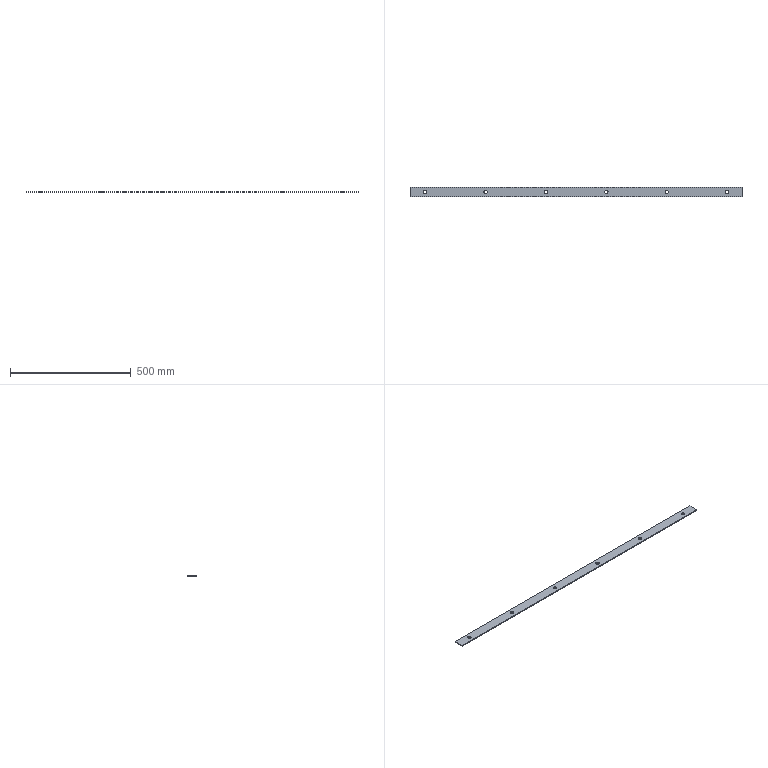Part | STEP file | Pressure plate 2_Default<As machined> | 1 solid | 18 faces | box 1374 x 40 x 4 mm | volume 216145 mm3 | cylinder 12 | plane 6 | commonest cylinder face diameters 14 x12
STEP:
#1=CARTESIAN_POINT('',(0.,0.,0.));
#2=DIRECTION('',(0.,0.,1.));
#3=DIRECTION('',(1.,0.,0.));
#4=AXIS2_PLACEMENT_3D('',#1,#2,#3);
#5=CARTESIAN_POINT('',(618.5,-541.136,4.));
#6=VERTEX_POINT('',#5);
#7=CARTESIAN_POINT('',(618.5,-541.136,0.));
#8=VERTEX_POINT('',#7);
#9=CARTESIAN_POINT('',(618.5,-541.136,4.));
#10=DIRECTION('',(0.,0.,-1.));
#11=VECTOR('',#10,1.);
#12=LINE('',#9,#11);
#13=CARTESIAN_POINT('',(625.5,-541.136,4.));
#14=DIRECTION('',(0.,0.,-1.));
#15=DIRECTION('',(-1.,0.,0.));
#16=AXIS2_PLACEMENT_3D('',#13,#14,#15);
#17=CYLINDRICAL_SURFACE('',#16,7.);
#18=CARTESIAN_POINT('',(6.283,0.));
#19=DIRECTION('',(0.,1.));
#20=VECTOR('',#19,1.);
#21=LINE('',#18,#20);
#22=(GEOMETRIC_REPRESENTATION_CONTEXT(2)PARAMETRIC_REPRESENTATION_CONTEXT()REPRESENTATION_CONTEXT('',''));
#23=DEFINITIONAL_REPRESENTATION('',(#21),#22);
#24=PCURVE('',#17,#23);
#25=CARTESIAN_POINT('',(625.5,-541.136,4.));
#26=DIRECTION('',(0.,0.,-1.));
#27=DIRECTION('',(-1.,0.,0.));
#28=AXIS2_PLACEMENT_3D('',#25,#26,#27);
#29=CYLINDRICAL_SURFACE('',#28,7.);
#30=CARTESIAN_POINT('',(0.,0.));
#31=DIRECTION('',(0.,1.));
#32=VECTOR('',#31,1.);
#33=LINE('',#30,#32);
#34=(GEOMETRIC_REPRESENTATION_CONTEXT(2)PARAMETRIC_REPRESENTATION_CONTEXT()REPRESENTATION_CONTEXT('',''));
#35=DEFINITIONAL_REPRESENTATION('',(#33),#34);
#36=PCURVE('',#29,#35);
#37=SURFACE_CURVE('',#12,(#24,#36),.PCURVE_S1.);
#38=EDGE_CURVE('',#6,#8,#37,.T.);
#39=ORIENTED_EDGE('',*,*,#38,.T.);
#40=CARTESIAN_POINT('',(632.5,-541.136,0.));
#41=VERTEX_POINT('',#40);
#42=CARTESIAN_POINT('',(625.5,-541.136,0.));
#43=DIRECTION('',(0.,0.,1.));
#44=DIRECTION('',(1.,0.,0.));
#45=AXIS2_PLACEMENT_3D('',#42,#43,#44);
#46=CIRCLE('',#45,7.);
#47=CARTESIAN_POINT('',(9.425,4.));
#48=DIRECTION('',(-1.,0.));
#49=VECTOR('',#48,1.);
#50=LINE('',#47,#49);
#51=(GEOMETRIC_REPRESENTATION_CONTEXT(2)PARAMETRIC_REPRESENTATION_CONTEXT()REPRESENTATION_CONTEXT('',''));
#52=DEFINITIONAL_REPRESENTATION('',(#50),#51);
#53=PCURVE('',#17,#52);
#54=CARTESIAN_POINT('',(0.,0.,0.));
#55=DIRECTION('',(0.,0.,1.));
#56=DIRECTION('',(1.,0.,0.));
#57=AXIS2_PLACEMENT_3D('',#54,#55,#56);
#58=PLANE('',#57);
#59=CARTESIAN_POINT('',(625.5,-541.136));
#60=DIRECTION('',(1.,0.));
#61=AXIS2_PLACEMENT_2D('',#59,#60);
#62=CIRCLE('',#61,7.);
#63=(GEOMETRIC_REPRESENTATION_CONTEXT(2)PARAMETRIC_REPRESENTATION_CONTEXT()REPRESENTATION_CONTEXT('',''));
#64=DEFINITIONAL_REPRESENTATION('',(#62),#63);
#65=PCURVE('',#58,#64);
#66=SURFACE_CURVE('',#46,(#53,#65),.PCURVE_S1.);
#67=EDGE_CURVE('',#8,#41,#66,.T.);
#68=ORIENTED_EDGE('',*,*,#67,.T.);
#69=CARTESIAN_POINT('',(632.5,-541.136,4.));
#70=VERTEX_POINT('',#69);
#71=CARTESIAN_POINT('',(632.5,-541.136,4.));
#72=DIRECTION('',(0.,0.,-1.));
#73=VECTOR('',#72,1.);
#74=LINE('',#71,#73);
#75=CARTESIAN_POINT('',(3.142,0.));
#76=DIRECTION('',(0.,1.));
#77=VECTOR('',#76,1.);
#78=LINE('',#75,#77);
#79=(GEOMETRIC_REPRESENTATION_CONTEXT(2)PARAMETRIC_REPRESENTATION_CONTEXT()REPRESENTATION_CONTEXT('',''));
#80=DEFINITIONAL_REPRESENTATION('',(#78),#79);
#81=PCURVE('',#17,#80);
#82=CARTESIAN_POINT('',(3.142,0.));
#83=DIRECTION('',(0.,1.));
#84=VECTOR('',#83,1.);
#85=LINE('',#82,#84);
#86=(GEOMETRIC_REPRESENTATION_CONTEXT(2)PARAMETRIC_REPRESENTATION_CONTEXT()REPRESENTATION_CONTEXT('',''));
#87=DEFINITIONAL_REPRESENTATION('',(#85),#86);
#88=PCURVE('',#29,#87);
#89=SURFACE_CURVE('',#74,(#81,#88),.PCURVE_S1.);
#90=EDGE_CURVE('',#70,#41,#89,.T.);
#91=ORIENTED_EDGE('',*,*,#90,.F.);
#92=CARTESIAN_POINT('',(625.5,-541.136,4.));
#93=DIRECTION('',(0.,0.,1.));
#94=DIRECTION('',(1.,0.,0.));
#95=AXIS2_PLACEMENT_3D('',#92,#93,#94);
#96=CIRCLE('',#95,7.);
#97=CARTESIAN_POINT('',(9.425,0.));
#98=DIRECTION('',(-1.,0.));
#99=VECTOR('',#98,1.);
#100=LINE('',#97,#99);
#101=(GEOMETRIC_REPRESENTATION_CONTEXT(2)PARAMETRIC_REPRESENTATION_CONTEXT()REPRESENTATION_CONTEXT('',''));
#102=DEFINITIONAL_REPRESENTATION('',(#100),#101);
#103=PCURVE('',#17,#102);
#104=CARTESIAN_POINT('',(0.,0.,4.));
#105=DIRECTION('',(0.,0.,1.));
#106=DIRECTION('',(1.,0.,0.));
#107=AXIS2_PLACEMENT_3D('',#104,#105,#106);
#108=PLANE('',#107);
#109=CARTESIAN_POINT('',(625.5,-541.136));
#110=DIRECTION('',(1.,0.));
#111=AXIS2_PLACEMENT_2D('',#109,#110);
#112=CIRCLE('',#111,7.);
#113=(GEOMETRIC_REPRESENTATION_CONTEXT(2)PARAMETRIC_REPRESENTATION_CONTEXT()REPRESENTATION_CONTEXT('',''));
#114=DEFINITIONAL_REPRESENTATION('',(#112),#113);
#115=PCURVE('',#108,#114);
#116=SURFACE_CURVE('',#96,(#103,#115),.PCURVE_S1.);
#117=EDGE_CURVE('',#6,#70,#116,.T.);
#118=ORIENTED_EDGE('',*,*,#117,.F.);
#119=EDGE_LOOP('',(#39,#68,#91,#118));
#120=FACE_BOUND('',#119,.F.);
#121=ADVANCED_FACE('',(#120),#17,.F.);
#122=CARTESIAN_POINT('',(368.5,-541.136,4.));
#123=VERTEX_POINT('',#122);
#124=CARTESIAN_POINT('',(368.5,-541.136,0.));
#125=VERTEX_POINT('',#124);
#126=CARTESIAN_POINT('',(368.5,-541.136,4.));
#127=DIRECTION('',(0.,0.,-1.));
#128=VECTOR('',#127,1.);
#129=LINE('',#126,#128);
#130=CARTESIAN_POINT('',(375.5,-541.136,4.));
#131=DIRECTION('',(0.,0.,-1.));
#132=DIRECTION('',(-1.,0.,0.));
#133=AXIS2_PLACEMENT_3D('',#130,#131,#132);
#134=CYLINDRICAL_SURFACE('',#133,7.);
#135=CARTESIAN_POINT('',(6.283,0.));
#136=DIRECTION('',(0.,1.));
#137=VECTOR('',#136,1.);
#138=LINE('',#135,#137);
#139=(GEOMETRIC_REPRESENTATION_CONTEXT(2)PARAMETRIC_REPRESENTATION_CONTEXT()REPRESENTATION_CONTEXT('',''));
#140=DEFINITIONAL_REPRESENTATION('',(#138),#139);
#141=PCURVE('',#134,#140);
#142=CARTESIAN_POINT('',(375.5,-541.136,4.));
#143=DIRECTION('',(0.,0.,-1.));
#144=DIRECTION('',(-1.,0.,0.));
#145=AXIS2_PLACEMENT_3D('',#142,#143,#144);
#146=CYLINDRICAL_SURFACE('',#145,7.);
#147=CARTESIAN_POINT('',(0.,0.));
#148=DIRECTION('',(0.,1.));
#149=VECTOR('',#148,1.);
#150=LINE('',#147,#149);
#151=(GEOMETRIC_REPRESENTATION_CONTEXT(2)PARAMETRIC_REPRESENTATION_CONTEXT()REPRESENTATION_CONTEXT('',''));
#152=DEFINITIONAL_REPRESENTATION('',(#150),#151);
#153=PCURVE('',#146,#152);
#154=SURFACE_CURVE('',#129,(#141,#153),.PCURVE_S1.);
#155=EDGE_CURVE('',#123,#125,#154,.T.);
#156=ORIENTED_EDGE('',*,*,#155,.T.);
#157=CARTESIAN_POINT('',(382.5,-541.136,0.));
#158=VERTEX_POINT('',#157);
#159=CARTESIAN_POINT('',(375.5,-541.136,0.));
#160=DIRECTION('',(0.,0.,1.));
#161=DIRECTION('',(1.,0.,0.));
#162=AXIS2_PLACEMENT_3D('',#159,#160,#161);
#163=CIRCLE('',#162,7.);
#164=CARTESIAN_POINT('',(9.425,4.));
#165=DIRECTION('',(-1.,0.));
#166=VECTOR('',#165,1.);
#167=LINE('',#164,#166);
#168=(GEOMETRIC_REPRESENTATION_CONTEXT(2)PARAMETRIC_REPRESENTATION_CONTEXT()REPRESENTATION_CONTEXT('',''));
#169=DEFINITIONAL_REPRESENTATION('',(#167),#168);
#170=PCURVE('',#134,#169);
#171=CARTESIAN_POINT('',(375.5,-541.136));
#172=DIRECTION('',(1.,0.));
#173=AXIS2_PLACEMENT_2D('',#171,#172);
#174=CIRCLE('',#173,7.);
#175=(GEOMETRIC_REPRESENTATION_CONTEXT(2)PARAMETRIC_REPRESENTATION_CONTEXT()REPRESENTATION_CONTEXT('',''));
#176=DEFINITIONAL_REPRESENTATION('',(#174),#175);
#177=PCURVE('',#58,#176);
#178=SURFACE_CURVE('',#163,(#170,#177),.PCURVE_S1.);
#179=EDGE_CURVE('',#125,#158,#178,.T.);
#180=ORIENTED_EDGE('',*,*,#179,.T.);
#181=CARTESIAN_POINT('',(382.5,-541.136,4.));
#182=VERTEX_POINT('',#181);
#183=CARTESIAN_POINT('',(382.5,-541.136,4.));
#184=DIRECTION('',(0.,0.,-1.));
#185=VECTOR('',#184,1.);
#186=LINE('',#183,#185);
#187=CARTESIAN_POINT('',(3.142,0.));
#188=DIRECTION('',(0.,1.));
#189=VECTOR('',#188,1.);
#190=LINE('',#187,#189);
#191=(GEOMETRIC_REPRESENTATION_CONTEXT(2)PARAMETRIC_REPRESENTATION_CONTEXT()REPRESENTATION_CONTEXT('',''));
#192=DEFINITIONAL_REPRESENTATION('',(#190),#191);
#193=PCURVE('',#134,#192);
#194=CARTESIAN_POINT('',(3.142,0.));
#195=DIRECTION('',(0.,1.));
#196=VECTOR('',#195,1.);
#197=LINE('',#194,#196);
#198=(GEOMETRIC_REPRESENTATION_CONTEXT(2)PARAMETRIC_REPRESENTATION_CONTEXT()REPRESENTATION_CONTEXT('',''));
#199=DEFINITIONAL_REPRESENTATION('',(#197),#198);
#200=PCURVE('',#146,#199);
#201=SURFACE_CURVE('',#186,(#193,#200),.PCURVE_S1.);
#202=EDGE_CURVE('',#182,#158,#201,.T.);
#203=ORIENTED_EDGE('',*,*,#202,.F.);
#204=CARTESIAN_POINT('',(375.5,-541.136,4.));
#205=DIRECTION('',(0.,0.,1.));
#206=DIRECTION('',(1.,0.,0.));
#207=AXIS2_PLACEMENT_3D('',#204,#205,#206);
#208=CIRCLE('',#207,7.);
#209=CARTESIAN_POINT('',(9.425,0.));
#210=DIRECTION('',(-1.,0.));
#211=VECTOR('',#210,1.);
#212=LINE('',#209,#211);
#213=(GEOMETRIC_REPRESENTATION_CONTEXT(2)PARAMETRIC_REPRESENTATION_CONTEXT()REPRESENTATION_CONTEXT('',''));
#214=DEFINITIONAL_REPRESENTATION('',(#212),#213);
#215=PCURVE('',#134,#214);
#216=CARTESIAN_POINT('',(375.5,-541.136));
#217=DIRECTION('',(1.,0.));
#218=AXIS2_PLACEMENT_2D('',#216,#217);
#219=CIRCLE('',#218,7.);
#220=(GEOMETRIC_REPRESENTATION_CONTEXT(2)PARAMETRIC_REPRESENTATION_CONTEXT()REPRESENTATION_CONTEXT('',''));
#221=DEFINITIONAL_REPRESENTATION('',(#219),#220);
#222=PCURVE('',#108,#221);
#223=SURFACE_CURVE('',#208,(#215,#222),.PCURVE_S1.);
#224=EDGE_CURVE('',#123,#182,#223,.T.);
#225=ORIENTED_EDGE('',*,*,#224,.F.);
#226=EDGE_LOOP('',(#156,#180,#203,#225));
#227=FACE_BOUND('',#226,.F.);
#228=ADVANCED_FACE('',(#227),#134,.F.);
#229=CARTESIAN_POINT('',(118.5,-541.136,4.));
#230=VERTEX_POINT('',#229);
#231=CARTESIAN_POINT('',(118.5,-541.136,0.));
#232=VERTEX_POINT('',#231);
#233=CARTESIAN_POINT('',(118.5,-541.136,4.));
#234=DIRECTION('',(0.,0.,-1.));
#235=VECTOR('',#234,1.);
#236=LINE('',#233,#235);
#237=CARTESIAN_POINT('',(125.5,-541.136,4.));
#238=DIRECTION('',(0.,0.,-1.));
#239=DIRECTION('',(-1.,0.,0.));
#240=AXIS2_PLACEMENT_3D('',#237,#238,#239);
#241=CYLINDRICAL_SURFACE('',#240,7.);
#242=CARTESIAN_POINT('',(6.283,0.));
#243=DIRECTION('',(0.,1.));
#244=VECTOR('',#243,1.);
#245=LINE('',#242,#244);
#246=(GEOMETRIC_REPRESENTATION_CONTEXT(2)PARAMETRIC_REPRESENTATION_CONTEXT()REPRESENTATION_CONTEXT('',''));
#247=DEFINITIONAL_REPRESENTATION('',(#245),#246);
#248=PCURVE('',#241,#247);
#249=CARTESIAN_POINT('',(125.5,-541.136,4.));
#250=DIRECTION('',(0.,0.,-1.));
#251=DIRECTION('',(-1.,0.,0.));
#252=AXIS2_PLACEMENT_3D('',#249,#250,#251);
#253=CYLINDRICAL_SURFACE('',#252,7.);
#254=CARTESIAN_POINT('',(0.,0.));
#255=DIRECTION('',(0.,1.));
#256=VECTOR('',#255,1.);
#257=LINE('',#254,#256);
#258=(GEOMETRIC_REPRESENTATION_CONTEXT(2)PARAMETRIC_REPRESENTATION_CONTEXT()REPRESENTATION_CONTEXT('',''));
#259=DEFINITIONAL_REPRESENTATION('',(#257),#258);
#260=PCURVE('',#253,#259);
#261=SURFACE_CURVE('',#236,(#248,#260),.PCURVE_S1.);
#262=EDGE_CURVE('',#230,#232,#261,.T.);
#263=ORIENTED_EDGE('',*,*,#262,.T.);
#264=CARTESIAN_POINT('',(132.5,-541.136,0.));
#265=VERTEX_POINT('',#264);
#266=CARTESIAN_POINT('',(125.5,-541.136,0.));
#267=DIRECTION('',(0.,0.,1.));
#268=DIRECTION('',(1.,0.,0.));
#269=AXIS2_PLACEMENT_3D('',#266,#267,#268);
#270=CIRCLE('',#269,7.);
#271=CARTESIAN_POINT('',(9.425,4.));
#272=DIRECTION('',(-1.,0.));
#273=VECTOR('',#272,1.);
#274=LINE('',#271,#273);
#275=(GEOMETRIC_REPRESENTATION_CONTEXT(2)PARAMETRIC_REPRESENTATION_CONTEXT()REPRESENTATION_CONTEXT('',''));
#276=DEFINITIONAL_REPRESENTATION('',(#274),#275);
#277=PCURVE('',#241,#276);
#278=CARTESIAN_POINT('',(125.5,-541.136));
#279=DIRECTION('',(1.,0.));
#280=AXIS2_PLACEMENT_2D('',#278,#279);
#281=CIRCLE('',#280,7.);
#282=(GEOMETRIC_REPRESENTATION_CONTEXT(2)PARAMETRIC_REPRESENTATION_CONTEXT()REPRESENTATION_CONTEXT('',''));
#283=DEFINITIONAL_REPRESENTATION('',(#281),#282);
#284=PCURVE('',#58,#283);
#285=SURFACE_CURVE('',#270,(#277,#284),.PCURVE_S1.);
#286=EDGE_CURVE('',#232,#265,#285,.T.);
#287=ORIENTED_EDGE('',*,*,#286,.T.);
#288=CARTESIAN_POINT('',(132.5,-541.136,4.));
#289=VERTEX_POINT('',#288);
#290=CARTESIAN_POINT('',(132.5,-541.136,4.));
#291=DIRECTION('',(0.,0.,-1.));
#292=VECTOR('',#291,1.);
#293=LINE('',#290,#292);
#294=CARTESIAN_POINT('',(3.142,0.));
#295=DIRECTION('',(0.,1.));
#296=VECTOR('',#295,1.);
#297=LINE('',#294,#296);
#298=(GEOMETRIC_REPRESENTATION_CONTEXT(2)PARAMETRIC_REPRESENTATION_CONTEXT()REPRESENTATION_CONTEXT('',''));
#299=DEFINITIONAL_REPRESENTATION('',(#297),#298);
#300=PCURVE('',#241,#299);
#301=CARTESIAN_POINT('',(3.142,0.));
#302=DIRECTION('',(0.,1.));
#303=VECTOR('',#302,1.);
#304=LINE('',#301,#303);
#305=(GEOMETRIC_REPRESENTATION_CONTEXT(2)PARAMETRIC_REPRESENTATION_CONTEXT()REPRESENTATION_CONTEXT('',''));
#306=DEFINITIONAL_REPRESENTATION('',(#304),#305);
#307=PCURVE('',#253,#306);
#308=SURFACE_CURVE('',#293,(#300,#307),.PCURVE_S1.);
#309=EDGE_CURVE('',#289,#265,#308,.T.);
#310=ORIENTED_EDGE('',*,*,#309,.F.);
#311=CARTESIAN_POINT('',(125.5,-541.136,4.));
#312=DIRECTION('',(0.,0.,1.));
#313=DIRECTION('',(1.,0.,0.));
#314=AXIS2_PLACEMENT_3D('',#311,#312,#313);
#315=CIRCLE('',#314,7.);
#316=CARTESIAN_POINT('',(9.425,0.));
#317=DIRECTION('',(-1.,0.));
#318=VECTOR('',#317,1.);
#319=LINE('',#316,#318);
#320=(GEOMETRIC_REPRESENTATION_CONTEXT(2)PARAMETRIC_REPRESENTATION_CONTEXT()REPRESENTATION_CONTEXT('',''));
#321=DEFINITIONAL_REPRESENTATION('',(#319),#320);
#322=PCURVE('',#241,#321);
#323=CARTESIAN_POINT('',(125.5,-541.136));
#324=DIRECTION('',(1.,0.));
#325=AXIS2_PLACEMENT_2D('',#323,#324);
#326=CIRCLE('',#325,7.);
#327=(GEOMETRIC_REPRESENTATION_CONTEXT(2)PARAMETRIC_REPRESENTATION_CONTEXT()REPRESENTATION_CONTEXT('',''));
#328=DEFINITIONAL_REPRESENTATION('',(#326),#327);
#329=PCURVE('',#108,#328);
#330=SURFACE_CURVE('',#315,(#322,#329),.PCURVE_S1.);
#331=EDGE_CURVE('',#230,#289,#330,.T.);
#332=ORIENTED_EDGE('',*,*,#331,.F.);
#333=EDGE_LOOP('',(#263,#287,#310,#332));
#334=FACE_BOUND('',#333,.F.);
#335=ADVANCED_FACE('',(#334),#241,.F.);
#336=CARTESIAN_POINT('',(-131.5,-541.136,4.));
#337=VERTEX_POINT('',#336);
#338=CARTESIAN_POINT('',(-131.5,-541.136,0.));
#339=VERTEX_POINT('',#338);
#340=CARTESIAN_POINT('',(-131.5,-541.136,4.));
#341=DIRECTION('',(0.,0.,-1.));
#342=VECTOR('',#341,1.);
#343=LINE('',#340,#342);
#344=CARTESIAN_POINT('',(-124.5,-541.136,4.));
#345=DIRECTION('',(0.,0.,-1.));
#346=DIRECTION('',(-1.,0.,0.));
#347=AXIS2_PLACEMENT_3D('',#344,#345,#346);
#348=CYLINDRICAL_SURFACE('',#347,7.);
#349=CARTESIAN_POINT('',(6.283,0.));
#350=DIRECTION('',(0.,1.));
#351=VECTOR('',#350,1.);
#352=LINE('',#349,#351);
#353=(GEOMETRIC_REPRESENTATION_CONTEXT(2)PARAMETRIC_REPRESENTATION_CONTEXT()REPRESENTATION_CONTEXT('',''));
#354=DEFINITIONAL_REPRESENTATION('',(#352),#353);
#355=PCURVE('',#348,#354);
#356=CARTESIAN_POINT('',(-124.5,-541.136,4.));
#357=DIRECTION('',(0.,0.,-1.));
#358=DIRECTION('',(-1.,0.,0.));
#359=AXIS2_PLACEMENT_3D('',#356,#357,#358);
#360=CYLINDRICAL_SURFACE('',#359,7.);
#361=CARTESIAN_POINT('',(0.,0.));
#362=DIRECTION('',(0.,1.));
#363=VECTOR('',#362,1.);
#364=LINE('',#361,#363);
#365=(GEOMETRIC_REPRESENTATION_CONTEXT(2)PARAMETRIC_REPRESENTATION_CONTEXT()REPRESENTATION_CONTEXT('',''));
#366=DEFINITIONAL_REPRESENTATION('',(#364),#365);
#367=PCURVE('',#360,#366);
#368=SURFACE_CURVE('',#343,(#355,#367),.PCURVE_S1.);
#369=EDGE_CURVE('',#337,#339,#368,.T.);
#370=ORIENTED_EDGE('',*,*,#369,.T.);
#371=CARTESIAN_POINT('',(-117.5,-541.136,0.));
#372=VERTEX_POINT('',#371);
#373=CARTESIAN_POINT('',(-124.5,-541.136,0.));
#374=DIRECTION('',(0.,0.,1.));
#375=DIRECTION('',(1.,0.,0.));
#376=AXIS2_PLACEMENT_3D('',#373,#374,#375);
#377=CIRCLE('',#376,7.);
#378=CARTESIAN_POINT('',(9.425,4.));
#379=DIRECTION('',(-1.,0.));
#380=VECTOR('',#379,1.);
#381=LINE('',#378,#380);
#382=(GEOMETRIC_REPRESENTATION_CONTEXT(2)PARAMETRIC_REPRESENTATION_CONTEXT()REPRESENTATION_CONTEXT('',''));
#383=DEFINITIONAL_REPRESENTATION('',(#381),#382);
#384=PCURVE('',#348,#383);
#385=CARTESIAN_POINT('',(-124.5,-541.136));
#386=DIRECTION('',(1.,0.));
#387=AXIS2_PLACEMENT_2D('',#385,#386);
#388=CIRCLE('',#387,7.);
#389=(GEOMETRIC_REPRESENTATION_CONTEXT(2)PARAMETRIC_REPRESENTATION_CONTEXT()REPRESENTATION_CONTEXT('',''));
#390=DEFINITIONAL_REPRESENTATION('',(#388),#389);
#391=PCURVE('',#58,#390);
#392=SURFACE_CURVE('',#377,(#384,#391),.PCURVE_S1.);
#393=EDGE_CURVE('',#339,#372,#392,.T.);
#394=ORIENTED_EDGE('',*,*,#393,.T.);
#395=CARTESIAN_POINT('',(-117.5,-541.136,4.));
#396=VERTEX_POINT('',#395);
#397=CARTESIAN_POINT('',(-117.5,-541.136,4.));
#398=DIRECTION('',(0.,0.,-1.));
#399=VECTOR('',#398,1.);
#400=LINE('',#397,#399);
#401=CARTESIAN_POINT('',(3.142,0.));
#402=DIRECTION('',(0.,1.));
#403=VECTOR('',#402,1.);
#404=LINE('',#401,#403);
#405=(GEOMETRIC_REPRESENTATION_CONTEXT(2)PARAMETRIC_REPRESENTATION_CONTEXT()REPRESENTATION_CONTEXT('',''));
#406=DEFINITIONAL_REPRESENTATION('',(#404),#405);
#407=PCURVE('',#348,#406);
#408=CARTESIAN_POINT('',(3.142,0.));
#409=DIRECTION('',(0.,1.));
#410=VECTOR('',#409,1.);
#411=LINE('',#408,#410);
#412=(GEOMETRIC_REPRESENTATION_CONTEXT(2)PARAMETRIC_REPRESENTATION_CONTEXT()REPRESENTATION_CONTEXT('',''));
#413=DEFINITIONAL_REPRESENTATION('',(#411),#412);
#414=PCURVE('',#360,#413);
#415=SURFACE_CURVE('',#400,(#407,#414),.PCURVE_S1.);
#416=EDGE_CURVE('',#396,#372,#415,.T.);
#417=ORIENTED_EDGE('',*,*,#416,.F.);
#418=CARTESIAN_POINT('',(-124.5,-541.136,4.));
#419=DIRECTION('',(0.,0.,1.));
#420=DIRECTION('',(1.,0.,0.));
#421=AXIS2_PLACEMENT_3D('',#418,#419,#420);
#422=CIRCLE('',#421,7.);
#423=CARTESIAN_POINT('',(9.425,0.));
#424=DIRECTION('',(-1.,0.));
#425=VECTOR('',#424,1.);
#426=LINE('',#423,#425);
#427=(GEOMETRIC_REPRESENTATION_CONTEXT(2)PARAMETRIC_REPRESENTATION_CONTEXT()REPRESENTATION_CONTEXT('',''));
#428=DEFINITIONAL_REPRESENTATION('',(#426),#427);
#429=PCURVE('',#348,#428);
#430=CARTESIAN_POINT('',(-124.5,-541.136));
#431=DIRECTION('',(1.,0.));
#432=AXIS2_PLACEMENT_2D('',#430,#431);
#433=CIRCLE('',#432,7.);
#434=(GEOMETRIC_REPRESENTATION_CONTEXT(2)PARAMETRIC_REPRESENTATION_CONTEXT()REPRESENTATION_CONTEXT('',''));
#435=DEFINITIONAL_REPRESENTATION('',(#433),#434);
#436=PCURVE('',#108,#435);
#437=SURFACE_CURVE('',#422,(#429,#436),.PCURVE_S1.);
#438=EDGE_CURVE('',#337,#396,#437,.T.);
#439=ORIENTED_EDGE('',*,*,#438,.F.);
#440=EDGE_LOOP('',(#370,#394,#417,#439));
#441=FACE_BOUND('',#440,.F.);
#442=ADVANCED_FACE('',(#441),#348,.F.);
#443=CARTESIAN_POINT('',(-381.5,-541.136,4.));
#444=VERTEX_POINT('',#443);
#445=CARTESIAN_POINT('',(-381.5,-541.136,0.));
#446=VERTEX_POINT('',#445);
#447=CARTESIAN_POINT('',(-381.5,-541.136,4.));
#448=DIRECTION('',(0.,0.,-1.));
#449=VECTOR('',#448,1.);
#450=LINE('',#447,#449);
#451=CARTESIAN_POINT('',(-374.5,-541.136,4.));
#452=DIRECTION('',(0.,0.,-1.));
#453=DIRECTION('',(-1.,0.,0.));
#454=AXIS2_PLACEMENT_3D('',#451,#452,#453);
#455=CYLINDRICAL_SURFACE('',#454,7.);
#456=CARTESIAN_POINT('',(6.283,0.));
#457=DIRECTION('',(0.,1.));
#458=VECTOR('',#457,1.);
#459=LINE('',#456,#458);
#460=(GEOMETRIC_REPRESENTATION_CONTEXT(2)PARAMETRIC_REPRESENTATION_CONTEXT()REPRESENTATION_CONTEXT('',''));
#461=DEFINITIONAL_REPRESENTATION('',(#459),#460);
#462=PCURVE('',#455,#461);
#463=CARTESIAN_POINT('',(-374.5,-541.136,4.));
#464=DIRECTION('',(0.,0.,-1.));
#465=DIRECTION('',(-1.,0.,0.));
#466=AXIS2_PLACEMENT_3D('',#463,#464,#465);
#467=CYLINDRICAL_SURFACE('',#466,7.);
#468=CARTESIAN_POINT('',(0.,0.));
#469=DIRECTION('',(0.,1.));
#470=VECTOR('',#469,1.);
#471=LINE('',#468,#470);
#472=(GEOMETRIC_REPRESENTATION_CONTEXT(2)PARAMETRIC_REPRESENTATION_CONTEXT()REPRESENTATION_CONTEXT('',''));
#473=DEFINITIONAL_REPRESENTATION('',(#471),#472);
#474=PCURVE('',#467,#473);
#475=SURFACE_CURVE('',#450,(#462,#474),.PCURVE_S1.);
#476=EDGE_CURVE('',#444,#446,#475,.T.);
#477=ORIENTED_EDGE('',*,*,#476,.T.);
#478=CARTESIAN_POINT('',(-367.5,-541.136,0.));
#479=VERTEX_POINT('',#478);
#480=CARTESIAN_POINT('',(-374.5,-541.136,0.));
#481=DIRECTION('',(0.,0.,1.));
#482=DIRECTION('',(1.,0.,0.));
#483=AXIS2_PLACEMENT_3D('',#480,#481,#482);
#484=CIRCLE('',#483,7.);
#485=CARTESIAN_POINT('',(9.425,4.));
#486=DIRECTION('',(-1.,0.));
#487=VECTOR('',#486,1.);
#488=LINE('',#485,#487);
#489=(GEOMETRIC_REPRESENTATION_CONTEXT(2)PARAMETRIC_REPRESENTATION_CONTEXT()REPRESENTATION_CONTEXT('',''));
#490=DEFINITIONAL_REPRESENTATION('',(#488),#489);
#491=PCURVE('',#455,#490);
#492=CARTESIAN_POINT('',(-374.5,-541.136));
#493=DIRECTION('',(1.,0.));
#494=AXIS2_PLACEMENT_2D('',#492,#493);
#495=CIRCLE('',#494,7.);
#496=(GEOMETRIC_REPRESENTATION_CONTEXT(2)PARAMETRIC_REPRESENTATION_CONTEXT()REPRESENTATION_CONTEXT('',''));
#497=DEFINITIONAL_REPRESENTATION('',(#495),#496);
#498=PCURVE('',#58,#497);
#499=SURFACE_CURVE('',#484,(#491,#498),.PCURVE_S1.);
#500=EDGE_CURVE('',#446,#479,#499,.T.);
#501=ORIENTED_EDGE('',*,*,#500,.T.);
#502=CARTESIAN_POINT('',(-367.5,-541.136,4.));
#503=VERTEX_POINT('',#502);
#504=CARTESIAN_POINT('',(-367.5,-541.136,4.));
#505=DIRECTION('',(0.,0.,-1.));
#506=VECTOR('',#505,1.);
#507=LINE('',#504,#506);
#508=CARTESIAN_POINT('',(3.142,0.));
#509=DIRECTION('',(0.,1.));
#510=VECTOR('',#509,1.);
#511=LINE('',#508,#510);
#512=(GEOMETRIC_REPRESENTATION_CONTEXT(2)PARAMETRIC_REPRESENTATION_CONTEXT()REPRESENTATION_CONTEXT('',''));
#513=DEFINITIONAL_REPRESENTATION('',(#511),#512);
#514=PCURVE('',#455,#513);
#515=CARTESIAN_POINT('',(3.142,0.));
#516=DIRECTION('',(0.,1.));
#517=VECTOR('',#516,1.);
#518=LINE('',#515,#517);
#519=(GEOMETRIC_REPRESENTATION_CONTEXT(2)PARAMETRIC_REPRESENTATION_CONTEXT()REPRESENTATION_CONTEXT('',''));
#520=DEFINITIONAL_REPRESENTATION('',(#518),#519);
#521=PCURVE('',#467,#520);
#522=SURFACE_CURVE('',#507,(#514,#521),.PCURVE_S1.);
#523=EDGE_CURVE('',#503,#479,#522,.T.);
#524=ORIENTED_EDGE('',*,*,#523,.F.);
#525=CARTESIAN_POINT('',(-374.5,-541.136,4.));
#526=DIRECTION('',(0.,0.,1.));
#527=DIRECTION('',(1.,0.,0.));
#528=AXIS2_PLACEMENT_3D('',#525,#526,#527);
#529=CIRCLE('',#528,7.);
#530=CARTESIAN_POINT('',(9.425,0.));
#531=DIRECTION('',(-1.,0.));
#532=VECTOR('',#531,1.);
#533=LINE('',#530,#532);
#534=(GEOMETRIC_REPRESENTATION_CONTEXT(2)PARAMETRIC_REPRESENTATION_CONTEXT()REPRESENTATION_CONTEXT('',''));
#535=DEFINITIONAL_REPRESENTATION('',(#533),#534);
#536=PCURVE('',#455,#535);
#537=CARTESIAN_POINT('',(-374.5,-541.136));
#538=DIRECTION('',(1.,0.));
#539=AXIS2_PLACEMENT_2D('',#537,#538);
#540=CIRCLE('',#539,7.);
#541=(GEOMETRIC_REPRESENTATION_CONTEXT(2)PARAMETRIC_REPRESENTATION_CONTEXT()REPRESENTATION_CONTEXT('',''));
#542=DEFINITIONAL_REPRESENTATION('',(#540),#541);
#543=PCURVE('',#108,#542);
#544=SURFACE_CURVE('',#529,(#536,#543),.PCURVE_S1.);
#545=EDGE_CURVE('',#444,#503,#544,.T.);
#546=ORIENTED_EDGE('',*,*,#545,.F.);
#547=EDGE_LOOP('',(#477,#501,#524,#546));
#548=FACE_BOUND('',#547,.F.);
#549=ADVANCED_FACE('',(#548),#455,.F.);
#550=CARTESIAN_POINT('',(-631.,-541.136,4.));
#551=VERTEX_POINT('',#550);
#552=CARTESIAN_POINT('',(-631.,-541.136,0.));
#553=VERTEX_POINT('',#552);
#554=CARTESIAN_POINT('',(-631.,-541.136,4.));
#555=DIRECTION('',(0.,0.,-1.));
#556=VECTOR('',#555,1.);
#557=LINE('',#554,#556);
#558=CARTESIAN_POINT('',(-624.,-541.136,4.));
#559=DIRECTION('',(0.,0.,-1.));
#560=DIRECTION('',(-1.,0.,0.));
#561=AXIS2_PLACEMENT_3D('',#558,#559,#560);
#562=CYLINDRICAL_SURFACE('',#561,7.);
#563=CARTESIAN_POINT('',(6.283,0.));
#564=DIRECTION('',(0.,1.));
#565=VECTOR('',#564,1.);
#566=LINE('',#563,#565);
#567=(GEOMETRIC_REPRESENTATION_CONTEXT(2)PARAMETRIC_REPRESENTATION_CONTEXT()REPRESENTATION_CONTEXT('',''));
#568=DEFINITIONAL_REPRESENTATION('',(#566),#567);
#569=PCURVE('',#562,#568);
#570=CARTESIAN_POINT('',(-624.,-541.136,4.));
#571=DIRECTION('',(0.,0.,-1.));
#572=DIRECTION('',(-1.,0.,0.));
#573=AXIS2_PLACEMENT_3D('',#570,#571,#572);
#574=CYLINDRICAL_SURFACE('',#573,7.);
#575=CARTESIAN_POINT('',(0.,0.));
#576=DIRECTION('',(0.,1.));
#577=VECTOR('',#576,1.);
#578=LINE('',#575,#577);
#579=(GEOMETRIC_REPRESENTATION_CONTEXT(2)PARAMETRIC_REPRESENTATION_CONTEXT()REPRESENTATION_CONTEXT('',''));
#580=DEFINITIONAL_REPRESENTATION('',(#578),#579);
#581=PCURVE('',#574,#580);
#582=SURFACE_CURVE('',#557,(#569,#581),.PCURVE_S1.);
#583=EDGE_CURVE('',#551,#553,#582,.T.);
#584=ORIENTED_EDGE('',*,*,#583,.T.);
#585=CARTESIAN_POINT('',(-617.,-541.136,0.));
#586=VERTEX_POINT('',#585);
#587=CARTESIAN_POINT('',(-624.,-541.136,0.));
#588=DIRECTION('',(0.,0.,1.));
#589=DIRECTION('',(1.,0.,0.));
#590=AXIS2_PLACEMENT_3D('',#587,#588,#589);
#591=CIRCLE('',#590,7.);
#592=CARTESIAN_POINT('',(9.425,4.));
#593=DIRECTION('',(-1.,0.));
#594=VECTOR('',#593,1.);
#595=LINE('',#592,#594);
#596=(GEOMETRIC_REPRESENTATION_CONTEXT(2)PARAMETRIC_REPRESENTATION_CONTEXT()REPRESENTATION_CONTEXT('',''));
#597=DEFINITIONAL_REPRESENTATION('',(#595),#596);
#598=PCURVE('',#562,#597);
#599=CARTESIAN_POINT('',(-624.,-541.136));
#600=DIRECTION('',(1.,0.));
#601=AXIS2_PLACEMENT_2D('',#599,#600);
#602=CIRCLE('',#601,7.);
#603=(GEOMETRIC_REPRESENTATION_CONTEXT(2)PARAMETRIC_REPRESENTATION_CONTEXT()REPRESENTATION_CONTEXT('',''));
#604=DEFINITIONAL_REPRESENTATION('',(#602),#603);
#605=PCURVE('',#58,#604);
#606=SURFACE_CURVE('',#591,(#598,#605),.PCURVE_S1.);
#607=EDGE_CURVE('',#553,#586,#606,.T.);
#608=ORIENTED_EDGE('',*,*,#607,.T.);
#609=CARTESIAN_POINT('',(-617.,-541.136,4.));
#610=VERTEX_POINT('',#609);
#611=CARTESIAN_POINT('',(-617.,-541.136,4.));
#612=DIRECTION('',(0.,0.,-1.));
#613=VECTOR('',#612,1.);
#614=LINE('',#611,#613);
#615=CARTESIAN_POINT('',(3.142,0.));
#616=DIRECTION('',(0.,1.));
#617=VECTOR('',#616,1.);
#618=LINE('',#615,#617);
#619=(GEOMETRIC_REPRESENTATION_CONTEXT(2)PARAMETRIC_REPRESENTATION_CONTEXT()REPRESENTATION_CONTEXT('',''));
#620=DEFINITIONAL_REPRESENTATION('',(#618),#619);
#621=PCURVE('',#562,#620);
#622=CARTESIAN_POINT('',(3.142,0.));
#623=DIRECTION('',(0.,1.));
#624=VECTOR('',#623,1.);
#625=LINE('',#622,#624);
#626=(GEOMETRIC_REPRESENTATION_CONTEXT(2)PARAMETRIC_REPRESENTATION_CONTEXT()REPRESENTATION_CONTEXT('',''));
#627=DEFINITIONAL_REPRESENTATION('',(#625),#626);
#628=PCURVE('',#574,#627);
#629=SURFACE_CURVE('',#614,(#621,#628),.PCURVE_S1.);
#630=EDGE_CURVE('',#610,#586,#629,.T.);
#631=ORIENTED_EDGE('',*,*,#630,.F.);
#632=CARTESIAN_POINT('',(-624.,-541.136,4.));
#633=DIRECTION('',(0.,0.,1.));
#634=DIRECTION('',(1.,0.,0.));
#635=AXIS2_PLACEMENT_3D('',#632,#633,#634);
#636=CIRCLE('',#635,7.);
#637=CARTESIAN_POINT('',(9.425,0.));
#638=DIRECTION('',(-1.,0.));
#639=VECTOR('',#638,1.);
#640=LINE('',#637,#639);
#641=(GEOMETRIC_REPRESENTATION_CONTEXT(2)PARAMETRIC_REPRESENTATION_CONTEXT()REPRESENTATION_CONTEXT('',''));
#642=DEFINITIONAL_REPRESENTATION('',(#640),#641);
#643=PCURVE('',#562,#642);
#644=CARTESIAN_POINT('',(-624.,-541.136));
#645=DIRECTION('',(1.,0.));
#646=AXIS2_PLACEMENT_2D('',#644,#645);
#647=CIRCLE('',#646,7.);
#648=(GEOMETRIC_REPRESENTATION_CONTEXT(2)PARAMETRIC_REPRESENTATION_CONTEXT()REPRESENTATION_CONTEXT('',''));
#649=DEFINITIONAL_REPRESENTATION('',(#647),#648);
#650=PCURVE('',#108,#649);
#651=SURFACE_CURVE('',#636,(#643,#650),.PCURVE_S1.);
#652=EDGE_CURVE('',#551,#610,#651,.T.);
#653=ORIENTED_EDGE('',*,*,#652,.F.);
#654=EDGE_LOOP('',(#584,#608,#631,#653));
#655=FACE_BOUND('',#654,.F.);
#656=ADVANCED_FACE('',(#655),#562,.F.);
#657=CARTESIAN_POINT('',(-687.,-521.136,0.));
#658=VERTEX_POINT('',#657);
#659=CARTESIAN_POINT('',(687.,-521.136,0.));
#660=VERTEX_POINT('',#659);
#661=CARTESIAN_POINT('',(0.,-521.136,0.));
#662=DIRECTION('',(1.,0.,0.));
#663=VECTOR('',#662,1.);
#664=LINE('',#661,#663);
#665=CARTESIAN_POINT('',(0.,-521.136,4.));
#666=DIRECTION('',(0.,1.,0.));
#667=DIRECTION('',(-1.,0.,0.));
#668=AXIS2_PLACEMENT_3D('',#665,#666,#667);
#669=PLANE('',#668);
#670=CARTESIAN_POINT('',(0.,-4.));
#671=DIRECTION('',(-1.,0.));
#672=VECTOR('',#671,1.);
#673=LINE('',#670,#672);
#674=(GEOMETRIC_REPRESENTATION_CONTEXT(2)PARAMETRIC_REPRESENTATION_CONTEXT()REPRESENTATION_CONTEXT('',''));
#675=DEFINITIONAL_REPRESENTATION('',(#673),#674);
#676=PCURVE('',#669,#675);
#677=CARTESIAN_POINT('',(0.,-521.136));
#678=DIRECTION('',(1.,0.));
#679=VECTOR('',#678,1.);
#680=LINE('',#677,#679);
#681=(GEOMETRIC_REPRESENTATION_CONTEXT(2)PARAMETRIC_REPRESENTATION_CONTEXT()REPRESENTATION_CONTEXT('',''));
#682=DEFINITIONAL_REPRESENTATION('',(#680),#681);
#683=PCURVE('',#58,#682);
#684=SURFACE_CURVE('',#664,(#676,#683),.PCURVE_S1.);
#685=EDGE_CURVE('',#658,#660,#684,.T.);
#686=ORIENTED_EDGE('',*,*,#685,.F.);
#687=CARTESIAN_POINT('',(-687.,-521.136,4.));
#688=VERTEX_POINT('',#687);
#689=CARTESIAN_POINT('',(-687.,-521.136,4.));
#690=DIRECTION('',(0.,0.,-1.));
#691=VECTOR('',#690,1.);
#692=LINE('',#689,#691);
#693=CARTESIAN_POINT('',(687.,0.));
#694=DIRECTION('',(0.,-1.));
#695=VECTOR('',#694,1.);
#696=LINE('',#693,#695);
#697=(GEOMETRIC_REPRESENTATION_CONTEXT(2)PARAMETRIC_REPRESENTATION_CONTEXT()REPRESENTATION_CONTEXT('',''));
#698=DEFINITIONAL_REPRESENTATION('',(#696),#697);
#699=PCURVE('',#669,#698);
#700=CARTESIAN_POINT('',(-687.,0.,4.));
#701=DIRECTION('',(1.,0.,0.));
#702=DIRECTION('',(0.,1.,0.));
#703=AXIS2_PLACEMENT_3D('',#700,#701,#702);
#704=PLANE('',#703);
#705=CARTESIAN_POINT('',(-521.136,0.));
#706=DIRECTION('',(0.,-1.));
#707=VECTOR('',#706,1.);
#708=LINE('',#705,#707);
#709=(GEOMETRIC_REPRESENTATION_CONTEXT(2)PARAMETRIC_REPRESENTATION_CONTEXT()REPRESENTATION_CONTEXT('',''));
#710=DEFINITIONAL_REPRESENTATION('',(#708),#709);
#711=PCURVE('',#704,#710);
#712=SURFACE_CURVE('',#692,(#699,#711),.PCURVE_S1.);
#713=EDGE_CURVE('',#688,#658,#712,.T.);
#714=ORIENTED_EDGE('',*,*,#713,.F.);
#715=CARTESIAN_POINT('',(687.,-521.136,4.));
#716=VERTEX_POINT('',#715);
#717=CARTESIAN_POINT('',(0.,-521.136,4.));
#718=DIRECTION('',(1.,0.,0.));
#719=VECTOR('',#718,1.);
#720=LINE('',#717,#719);
#721=CARTESIAN_POINT('',(0.,0.));
#722=DIRECTION('',(-1.,0.));
#723=VECTOR('',#722,1.);
#724=LINE('',#721,#723);
#725=(GEOMETRIC_REPRESENTATION_CONTEXT(2)PARAMETRIC_REPRESENTATION_CONTEXT()REPRESENTATION_CONTEXT('',''));
#726=DEFINITIONAL_REPRESENTATION('',(#724),#725);
#727=PCURVE('',#669,#726);
#728=CARTESIAN_POINT('',(0.,-521.136));
#729=DIRECTION('',(1.,0.));
#730=VECTOR('',#729,1.);
#731=LINE('',#728,#730);
#732=(GEOMETRIC_REPRESENTATION_CONTEXT(2)PARAMETRIC_REPRESENTATION_CONTEXT()REPRESENTATION_CONTEXT('',''));
#733=DEFINITIONAL_REPRESENTATION('',(#731),#732);
#734=PCURVE('',#108,#733);
#735=SURFACE_CURVE('',#720,(#727,#734),.PCURVE_S1.);
#736=EDGE_CURVE('',#688,#716,#735,.T.);
#737=ORIENTED_EDGE('',*,*,#736,.T.);
#738=CARTESIAN_POINT('',(687.,-521.136,4.));
#739=DIRECTION('',(0.,0.,-1.));
#740=VECTOR('',#739,1.);
#741=LINE('',#738,#740);
#742=CARTESIAN_POINT('',(-687.,0.));
#743=DIRECTION('',(0.,-1.));
#744=VECTOR('',#743,1.);
#745=LINE('',#742,#744);
#746=(GEOMETRIC_REPRESENTATION_CONTEXT(2)PARAMETRIC_REPRESENTATION_CONTEXT()REPRESENTATION_CONTEXT('',''));
#747=DEFINITIONAL_REPRESENTATION('',(#745),#746);
#748=PCURVE('',#669,#747);
#749=CARTESIAN_POINT('',(687.,0.,4.));
#750=DIRECTION('',(1.,0.,0.));
#751=DIRECTION('',(0.,0.,-1.));
#752=AXIS2_PLACEMENT_3D('',#749,#750,#751);
#753=PLANE('',#752);
#754=CARTESIAN_POINT('',(0.,-521.136));
#755=DIRECTION('',(1.,0.));
#756=VECTOR('',#755,1.);
#757=LINE('',#754,#756);
#758=(GEOMETRIC_REPRESENTATION_CONTEXT(2)PARAMETRIC_REPRESENTATION_CONTEXT()REPRESENTATION_CONTEXT('',''));
#759=DEFINITIONAL_REPRESENTATION('',(#757),#758);
#760=PCURVE('',#753,#759);
#761=SURFACE_CURVE('',#741,(#748,#760),.PCURVE_S1.);
#762=EDGE_CURVE('',#716,#660,#761,.T.);
#763=ORIENTED_EDGE('',*,*,#762,.T.);
#764=EDGE_LOOP('',(#686,#714,#737,#763));
#765=FACE_BOUND('',#764,.T.);
#766=ADVANCED_FACE('',(#765),#669,.T.);
#767=CARTESIAN_POINT('',(-687.,-561.136,0.));
#768=VERTEX_POINT('',#767);
#769=CARTESIAN_POINT('',(-687.,0.,0.));
#770=DIRECTION('',(0.,-1.,0.));
#771=VECTOR('',#770,1.);
#772=LINE('',#769,#771);
#773=CARTESIAN_POINT('',(0.,-4.));
#774=DIRECTION('',(-1.,0.));
#775=VECTOR('',#774,1.);
#776=LINE('',#773,#775);
#777=(GEOMETRIC_REPRESENTATION_CONTEXT(2)PARAMETRIC_REPRESENTATION_CONTEXT()REPRESENTATION_CONTEXT('',''));
#778=DEFINITIONAL_REPRESENTATION('',(#776),#777);
#779=PCURVE('',#704,#778);
#780=CARTESIAN_POINT('',(-687.,0.));
#781=DIRECTION('',(0.,-1.));
#782=VECTOR('',#781,1.);
#783=LINE('',#780,#782);
#784=(GEOMETRIC_REPRESENTATION_CONTEXT(2)PARAMETRIC_REPRESENTATION_CONTEXT()REPRESENTATION_CONTEXT('',''));
#785=DEFINITIONAL_REPRESENTATION('',(#783),#784);
#786=PCURVE('',#58,#785);
#787=SURFACE_CURVE('',#772,(#779,#786),.PCURVE_S1.);
#788=EDGE_CURVE('',#658,#768,#787,.T.);
#789=ORIENTED_EDGE('',*,*,#788,.T.);
#790=CARTESIAN_POINT('',(-687.,-561.136,4.));
#791=VERTEX_POINT('',#790);
#792=CARTESIAN_POINT('',(-687.,-561.136,4.));
#793=DIRECTION('',(0.,0.,-1.));
#794=VECTOR('',#793,1.);
#795=LINE('',#792,#794);
#796=CARTESIAN_POINT('',(-561.136,0.));
#797=DIRECTION('',(0.,-1.));
#798=VECTOR('',#797,1.);
#799=LINE('',#796,#798);
#800=(GEOMETRIC_REPRESENTATION_CONTEXT(2)PARAMETRIC_REPRESENTATION_CONTEXT()REPRESENTATION_CONTEXT('',''));
#801=DEFINITIONAL_REPRESENTATION('',(#799),#800);
#802=PCURVE('',#704,#801);
#803=CARTESIAN_POINT('',(0.,-561.136,4.));
#804=DIRECTION('',(0.,1.,0.));
#805=DIRECTION('',(0.,0.,1.));
#806=AXIS2_PLACEMENT_3D('',#803,#804,#805);
#807=PLANE('',#806);
#808=CARTESIAN_POINT('',(0.,-687.));
#809=DIRECTION('',(-1.,0.));
#810=VECTOR('',#809,1.);
#811=LINE('',#808,#810);
#812=(GEOMETRIC_REPRESENTATION_CONTEXT(2)PARAMETRIC_REPRESENTATION_CONTEXT()REPRESENTATION_CONTEXT('',''));
#813=DEFINITIONAL_REPRESENTATION('',(#811),#812);
#814=PCURVE('',#807,#813);
#815=SURFACE_CURVE('',#795,(#802,#814),.PCURVE_S1.);
#816=EDGE_CURVE('',#791,#768,#815,.T.);
#817=ORIENTED_EDGE('',*,*,#816,.F.);
#818=CARTESIAN_POINT('',(-687.,0.,4.));
#819=DIRECTION('',(0.,-1.,0.));
#820=VECTOR('',#819,1.);
#821=LINE('',#818,#820);
#822=CARTESIAN_POINT('',(0.,0.));
#823=DIRECTION('',(-1.,0.));
#824=VECTOR('',#823,1.);
#825=LINE('',#822,#824);
#826=(GEOMETRIC_REPRESENTATION_CONTEXT(2)PARAMETRIC_REPRESENTATION_CONTEXT()REPRESENTATION_CONTEXT('',''));
#827=DEFINITIONAL_REPRESENTATION('',(#825),#826);
#828=PCURVE('',#704,#827);
#829=CARTESIAN_POINT('',(-687.,0.));
#830=DIRECTION('',(0.,-1.));
#831=VECTOR('',#830,1.);
#832=LINE('',#829,#831);
#833=(GEOMETRIC_REPRESENTATION_CONTEXT(2)PARAMETRIC_REPRESENTATION_CONTEXT()REPRESENTATION_CONTEXT('',''));
#834=DEFINITIONAL_REPRESENTATION('',(#832),#833);
#835=PCURVE('',#108,#834);
#836=SURFACE_CURVE('',#821,(#828,#835),.PCURVE_S1.);
#837=EDGE_CURVE('',#688,#791,#836,.T.);
#838=ORIENTED_EDGE('',*,*,#837,.F.);
#839=ORIENTED_EDGE('',*,*,#713,.T.);
#840=EDGE_LOOP('',(#789,#817,#838,#839));
#841=FACE_BOUND('',#840,.T.);
#842=ADVANCED_FACE('',(#841),#704,.F.);
#843=CARTESIAN_POINT('',(687.,-561.136,0.));
#844=VERTEX_POINT('',#843);
#845=CARTESIAN_POINT('',(0.,-561.136,0.));
#846=DIRECTION('',(1.,0.,0.));
#847=VECTOR('',#846,1.);
#848=LINE('',#845,#847);
#849=CARTESIAN_POINT('',(-4.,0.));
#850=DIRECTION('',(0.,1.));
#851=VECTOR('',#850,1.);
#852=LINE('',#849,#851);
#853=(GEOMETRIC_REPRESENTATION_CONTEXT(2)PARAMETRIC_REPRESENTATION_CONTEXT()REPRESENTATION_CONTEXT('',''));
#854=DEFINITIONAL_REPRESENTATION('',(#852),#853);
#855=PCURVE('',#807,#854);
#856=CARTESIAN_POINT('',(0.,-561.136));
#857=DIRECTION('',(1.,0.));
#858=VECTOR('',#857,1.);
#859=LINE('',#856,#858);
#860=(GEOMETRIC_REPRESENTATION_CONTEXT(2)PARAMETRIC_REPRESENTATION_CONTEXT()REPRESENTATION_CONTEXT('',''));
#861=DEFINITIONAL_REPRESENTATION('',(#859),#860);
#862=PCURVE('',#58,#861);
#863=SURFACE_CURVE('',#848,(#855,#862),.PCURVE_S1.);
#864=EDGE_CURVE('',#768,#844,#863,.T.);
#865=ORIENTED_EDGE('',*,*,#864,.T.);
#866=CARTESIAN_POINT('',(687.,-561.136,4.));
#867=VERTEX_POINT('',#866);
#868=CARTESIAN_POINT('',(687.,-561.136,4.));
#869=DIRECTION('',(0.,0.,-1.));
#870=VECTOR('',#869,1.);
#871=LINE('',#868,#870);
#872=CARTESIAN_POINT('',(0.,687.));
#873=DIRECTION('',(-1.,0.));
#874=VECTOR('',#873,1.);
#875=LINE('',#872,#874);
#876=(GEOMETRIC_REPRESENTATION_CONTEXT(2)PARAMETRIC_REPRESENTATION_CONTEXT()REPRESENTATION_CONTEXT('',''));
#877=DEFINITIONAL_REPRESENTATION('',(#875),#876);
#878=PCURVE('',#807,#877);
#879=CARTESIAN_POINT('',(0.,-561.136));
#880=DIRECTION('',(1.,0.));
#881=VECTOR('',#880,1.);
#882=LINE('',#879,#881);
#883=(GEOMETRIC_REPRESENTATION_CONTEXT(2)PARAMETRIC_REPRESENTATION_CONTEXT()REPRESENTATION_CONTEXT('',''));
#884=DEFINITIONAL_REPRESENTATION('',(#882),#883);
#885=PCURVE('',#753,#884);
#886=SURFACE_CURVE('',#871,(#878,#885),.PCURVE_S1.);
#887=EDGE_CURVE('',#867,#844,#886,.T.);
#888=ORIENTED_EDGE('',*,*,#887,.F.);
#889=CARTESIAN_POINT('',(0.,-561.136,4.));
#890=DIRECTION('',(1.,0.,0.));
#891=VECTOR('',#890,1.);
#892=LINE('',#889,#891);
#893=CARTESIAN_POINT('',(0.,0.));
#894=DIRECTION('',(0.,1.));
#895=VECTOR('',#894,1.);
#896=LINE('',#893,#895);
#897=(GEOMETRIC_REPRESENTATION_CONTEXT(2)PARAMETRIC_REPRESENTATION_CONTEXT()REPRESENTATION_CONTEXT('',''));
#898=DEFINITIONAL_REPRESENTATION('',(#896),#897);
#899=PCURVE('',#807,#898);
#900=CARTESIAN_POINT('',(0.,-561.136));
#901=DIRECTION('',(1.,0.));
#902=VECTOR('',#901,1.);
#903=LINE('',#900,#902);
#904=(GEOMETRIC_REPRESENTATION_CONTEXT(2)PARAMETRIC_REPRESENTATION_CONTEXT()REPRESENTATION_CONTEXT('',''));
#905=DEFINITIONAL_REPRESENTATION('',(#903),#904);
#906=PCURVE('',#108,#905);
#907=SURFACE_CURVE('',#892,(#899,#906),.PCURVE_S1.);
#908=EDGE_CURVE('',#791,#867,#907,.T.);
#909=ORIENTED_EDGE('',*,*,#908,.F.);
#910=ORIENTED_EDGE('',*,*,#816,.T.);
#911=EDGE_LOOP('',(#865,#888,#909,#910));
#912=FACE_BOUND('',#911,.T.);
#913=ADVANCED_FACE('',(#912),#807,.F.);
#914=CARTESIAN_POINT('',(-624.,-541.136,0.));
#915=DIRECTION('',(0.,0.,1.));
#916=DIRECTION('',(1.,0.,0.));
#917=AXIS2_PLACEMENT_3D('',#914,#915,#916);
#918=CIRCLE('',#917,7.);
#919=CARTESIAN_POINT('',(3.142,4.));
#920=DIRECTION('',(-1.,0.));
#921=VECTOR('',#920,1.);
#922=LINE('',#919,#921);
#923=(GEOMETRIC_REPRESENTATION_CONTEXT(2)PARAMETRIC_REPRESENTATION_CONTEXT()REPRESENTATION_CONTEXT('',''));
#924=DEFINITIONAL_REPRESENTATION('',(#922),#923);
#925=PCURVE('',#574,#924);
#926=CARTESIAN_POINT('',(-624.,-541.136));
#927=DIRECTION('',(1.,0.));
#928=AXIS2_PLACEMENT_2D('',#926,#927);
#929=CIRCLE('',#928,7.);
#930=(GEOMETRIC_REPRESENTATION_CONTEXT(2)PARAMETRIC_REPRESENTATION_CONTEXT()REPRESENTATION_CONTEXT('',''));
#931=DEFINITIONAL_REPRESENTATION('',(#929),#930);
#932=PCURVE('',#58,#931);
#933=SURFACE_CURVE('',#918,(#925,#932),.PCURVE_S1.);
#934=EDGE_CURVE('',#586,#553,#933,.T.);
#935=ORIENTED_EDGE('',*,*,#934,.T.);
#936=ORIENTED_EDGE('',*,*,#583,.F.);
#937=CARTESIAN_POINT('',(-624.,-541.136,4.));
#938=DIRECTION('',(0.,0.,1.));
#939=DIRECTION('',(1.,0.,0.));
#940=AXIS2_PLACEMENT_3D('',#937,#938,#939);
#941=CIRCLE('',#940,7.);
#942=CARTESIAN_POINT('',(3.142,0.));
#943=DIRECTION('',(-1.,0.));
#944=VECTOR('',#943,1.);
#945=LINE('',#942,#944);
#946=(GEOMETRIC_REPRESENTATION_CONTEXT(2)PARAMETRIC_REPRESENTATION_CONTEXT()REPRESENTATION_CONTEXT('',''));
#947=DEFINITIONAL_REPRESENTATION('',(#945),#946);
#948=PCURVE('',#574,#947);
#949=CARTESIAN_POINT('',(-624.,-541.136));
#950=DIRECTION('',(1.,0.));
#951=AXIS2_PLACEMENT_2D('',#949,#950);
#952=CIRCLE('',#951,7.);
#953=(GEOMETRIC_REPRESENTATION_CONTEXT(2)PARAMETRIC_REPRESENTATION_CONTEXT()REPRESENTATION_CONTEXT('',''));
#954=DEFINITIONAL_REPRESENTATION('',(#952),#953);
#955=PCURVE('',#108,#954);
#956=SURFACE_CURVE('',#941,(#948,#955),.PCURVE_S1.);
#957=EDGE_CURVE('',#610,#551,#956,.T.);
#958=ORIENTED_EDGE('',*,*,#957,.F.);
#959=ORIENTED_EDGE('',*,*,#630,.T.);
#960=EDGE_LOOP('',(#935,#936,#958,#959));
#961=FACE_BOUND('',#960,.F.);
#962=ADVANCED_FACE('',(#961),#574,.F.);
#963=CARTESIAN_POINT('',(-374.5,-541.136,0.));
#964=DIRECTION('',(0.,0.,1.));
#965=DIRECTION('',(1.,0.,0.));
#966=AXIS2_PLACEMENT_3D('',#963,#964,#965);
#967=CIRCLE('',#966,7.);
#968=CARTESIAN_POINT('',(3.142,4.));
#969=DIRECTION('',(-1.,0.));
#970=VECTOR('',#969,1.);
#971=LINE('',#968,#970);
#972=(GEOMETRIC_REPRESENTATION_CONTEXT(2)PARAMETRIC_REPRESENTATION_CONTEXT()REPRESENTATION_CONTEXT('',''));
#973=DEFINITIONAL_REPRESENTATION('',(#971),#972);
#974=PCURVE('',#467,#973);
#975=CARTESIAN_POINT('',(-374.5,-541.136));
#976=DIRECTION('',(1.,0.));
#977=AXIS2_PLACEMENT_2D('',#975,#976);
#978=CIRCLE('',#977,7.);
#979=(GEOMETRIC_REPRESENTATION_CONTEXT(2)PARAMETRIC_REPRESENTATION_CONTEXT()REPRESENTATION_CONTEXT('',''));
#980=DEFINITIONAL_REPRESENTATION('',(#978),#979);
#981=PCURVE('',#58,#980);
#982=SURFACE_CURVE('',#967,(#974,#981),.PCURVE_S1.);
#983=EDGE_CURVE('',#479,#446,#982,.T.);
#984=ORIENTED_EDGE('',*,*,#983,.T.);
#985=ORIENTED_EDGE('',*,*,#476,.F.);
#986=CARTESIAN_POINT('',(-374.5,-541.136,4.));
#987=DIRECTION('',(0.,0.,1.));
#988=DIRECTION('',(1.,0.,0.));
#989=AXIS2_PLACEMENT_3D('',#986,#987,#988);
#990=CIRCLE('',#989,7.);
#991=CARTESIAN_POINT('',(3.142,0.));
#992=DIRECTION('',(-1.,0.));
#993=VECTOR('',#992,1.);
#994=LINE('',#991,#993);
#995=(GEOMETRIC_REPRESENTATION_CONTEXT(2)PARAMETRIC_REPRESENTATION_CONTEXT()REPRESENTATION_CONTEXT('',''));
#996=DEFINITIONAL_REPRESENTATION('',(#994),#995);
#997=PCURVE('',#467,#996);
#998=CARTESIAN_POINT('',(-374.5,-541.136));
#999=DIRECTION('',(1.,0.));
#1000=AXIS2_PLACEMENT_2D('',#998,#999);
#1001=CIRCLE('',#1000,7.);
#1002=(GEOMETRIC_REPRESENTATION_CONTEXT(2)PARAMETRIC_REPRESENTATION_CONTEXT()REPRESENTATION_CONTEXT('',''));
#1003=DEFINITIONAL_REPRESENTATION('',(#1001),#1002);
#1004=PCURVE('',#108,#1003);
#1005=SURFACE_CURVE('',#990,(#997,#1004),.PCURVE_S1.);
#1006=EDGE_CURVE('',#503,#444,#1005,.T.);
#1007=ORIENTED_EDGE('',*,*,#1006,.F.);
#1008=ORIENTED_EDGE('',*,*,#523,.T.);
#1009=EDGE_LOOP('',(#984,#985,#1007,#1008));
#1010=FACE_BOUND('',#1009,.F.);
#1011=ADVANCED_FACE('',(#1010),#467,.F.);
#1012=CARTESIAN_POINT('',(-124.5,-541.136,0.));
#1013=DIRECTION('',(0.,0.,1.));
#1014=DIRECTION('',(1.,0.,0.));
#1015=AXIS2_PLACEMENT_3D('',#1012,#1013,#1014);
#1016=CIRCLE('',#1015,7.);
#1017=CARTESIAN_POINT('',(3.142,4.));
#1018=DIRECTION('',(-1.,0.));
#1019=VECTOR('',#1018,1.);
#1020=LINE('',#1017,#1019);
#1021=(GEOMETRIC_REPRESENTATION_CONTEXT(2)PARAMETRIC_REPRESENTATION_CONTEXT()REPRESENTATION_CONTEXT('',''));
#1022=DEFINITIONAL_REPRESENTATION('',(#1020),#1021);
#1023=PCURVE('',#360,#1022);
#1024=CARTESIAN_POINT('',(-124.5,-541.136));
#1025=DIRECTION('',(1.,0.));
#1026=AXIS2_PLACEMENT_2D('',#1024,#1025);
#1027=CIRCLE('',#1026,7.);
#1028=(GEOMETRIC_REPRESENTATION_CONTEXT(2)PARAMETRIC_REPRESENTATION_CONTEXT()REPRESENTATION_CONTEXT('',''));
#1029=DEFINITIONAL_REPRESENTATION('',(#1027),#1028);
#1030=PCURVE('',#58,#1029);
#1031=SURFACE_CURVE('',#1016,(#1023,#1030),.PCURVE_S1.);
#1032=EDGE_CURVE('',#372,#339,#1031,.T.);
#1033=ORIENTED_EDGE('',*,*,#1032,.T.);
#1034=ORIENTED_EDGE('',*,*,#369,.F.);
#1035=CARTESIAN_POINT('',(-124.5,-541.136,4.));
#1036=DIRECTION('',(0.,0.,1.));
#1037=DIRECTION('',(1.,0.,0.));
#1038=AXIS2_PLACEMENT_3D('',#1035,#1036,#1037);
#1039=CIRCLE('',#1038,7.);
#1040=CARTESIAN_POINT('',(3.142,0.));
#1041=DIRECTION('',(-1.,0.));
#1042=VECTOR('',#1041,1.);
#1043=LINE('',#1040,#1042);
#1044=(GEOMETRIC_REPRESENTATION_CONTEXT(2)PARAMETRIC_REPRESENTATION_CONTEXT()REPRESENTATION_CONTEXT('',''));
#1045=DEFINITIONAL_REPRESENTATION('',(#1043),#1044);
#1046=PCURVE('',#360,#1045);
#1047=CARTESIAN_POINT('',(-124.5,-541.136));
#1048=DIRECTION('',(1.,0.));
#1049=AXIS2_PLACEMENT_2D('',#1047,#1048);
#1050=CIRCLE('',#1049,7.);
#1051=(GEOMETRIC_REPRESENTATION_CONTEXT(2)PARAMETRIC_REPRESENTATION_CONTEXT()REPRESENTATION_CONTEXT('',''));
#1052=DEFINITIONAL_REPRESENTATION('',(#1050),#1051);
#1053=PCURVE('',#108,#1052);
#1054=SURFACE_CURVE('',#1039,(#1046,#1053),.PCURVE_S1.);
#1055=EDGE_CURVE('',#396,#337,#1054,.T.);
#1056=ORIENTED_EDGE('',*,*,#1055,.F.);
#1057=ORIENTED_EDGE('',*,*,#416,.T.);
#1058=EDGE_LOOP('',(#1033,#1034,#1056,#1057));
#1059=FACE_BOUND('',#1058,.F.);
#1060=ADVANCED_FACE('',(#1059),#360,.F.);
#1061=CARTESIAN_POINT('',(125.5,-541.136,0.));
#1062=DIRECTION('',(0.,0.,1.));
#1063=DIRECTION('',(1.,0.,0.));
#1064=AXIS2_PLACEMENT_3D('',#1061,#1062,#1063);
#1065=CIRCLE('',#1064,7.);
#1066=CARTESIAN_POINT('',(3.142,4.));
#1067=DIRECTION('',(-1.,0.));
#1068=VECTOR('',#1067,1.);
#1069=LINE('',#1066,#1068);
#1070=(GEOMETRIC_REPRESENTATION_CONTEXT(2)PARAMETRIC_REPRESENTATION_CONTEXT()REPRESENTATION_CONTEXT('',''));
#1071=DEFINITIONAL_REPRESENTATION('',(#1069),#1070);
#1072=PCURVE('',#253,#1071);
#1073=CARTESIAN_POINT('',(125.5,-541.136));
#1074=DIRECTION('',(1.,0.));
#1075=AXIS2_PLACEMENT_2D('',#1073,#1074);
#1076=CIRCLE('',#1075,7.);
#1077=(GEOMETRIC_REPRESENTATION_CONTEXT(2)PARAMETRIC_REPRESENTATION_CONTEXT()REPRESENTATION_CONTEXT('',''));
#1078=DEFINITIONAL_REPRESENTATION('',(#1076),#1077);
#1079=PCURVE('',#58,#1078);
#1080=SURFACE_CURVE('',#1065,(#1072,#1079),.PCURVE_S1.);
#1081=EDGE_CURVE('',#265,#232,#1080,.T.);
#1082=ORIENTED_EDGE('',*,*,#1081,.T.);
#1083=ORIENTED_EDGE('',*,*,#262,.F.);
#1084=CARTESIAN_POINT('',(125.5,-541.136,4.));
#1085=DIRECTION('',(0.,0.,1.));
#1086=DIRECTION('',(1.,0.,0.));
#1087=AXIS2_PLACEMENT_3D('',#1084,#1085,#1086);
#1088=CIRCLE('',#1087,7.);
#1089=CARTESIAN_POINT('',(3.142,0.));
#1090=DIRECTION('',(-1.,0.));
#1091=VECTOR('',#1090,1.);
#1092=LINE('',#1089,#1091);
#1093=(GEOMETRIC_REPRESENTATION_CONTEXT(2)PARAMETRIC_REPRESENTATION_CONTEXT()REPRESENTATION_CONTEXT('',''));
#1094=DEFINITIONAL_REPRESENTATION('',(#1092),#1093);
#1095=PCURVE('',#253,#1094);
#1096=CARTESIAN_POINT('',(125.5,-541.136));
#1097=DIRECTION('',(1.,0.));
#1098=AXIS2_PLACEMENT_2D('',#1096,#1097);
#1099=CIRCLE('',#1098,7.);
#1100=(GEOMETRIC_REPRESENTATION_CONTEXT(2)PARAMETRIC_REPRESENTATION_CONTEXT()REPRESENTATION_CONTEXT('',''));
#1101=DEFINITIONAL_REPRESENTATION('',(#1099),#1100);
#1102=PCURVE('',#108,#1101);
#1103=SURFACE_CURVE('',#1088,(#1095,#1102),.PCURVE_S1.);
#1104=EDGE_CURVE('',#289,#230,#1103,.T.);
#1105=ORIENTED_EDGE('',*,*,#1104,.F.);
#1106=ORIENTED_EDGE('',*,*,#309,.T.);
#1107=EDGE_LOOP('',(#1082,#1083,#1105,#1106));
#1108=FACE_BOUND('',#1107,.F.);
#1109=ADVANCED_FACE('',(#1108),#253,.F.);
#1110=CARTESIAN_POINT('',(375.5,-541.136,0.));
#1111=DIRECTION('',(0.,0.,1.));
#1112=DIRECTION('',(1.,0.,0.));
#1113=AXIS2_PLACEMENT_3D('',#1110,#1111,#1112);
#1114=CIRCLE('',#1113,7.);
#1115=CARTESIAN_POINT('',(3.142,4.));
#1116=DIRECTION('',(-1.,0.));
#1117=VECTOR('',#1116,1.);
#1118=LINE('',#1115,#1117);
#1119=(GEOMETRIC_REPRESENTATION_CONTEXT(2)PARAMETRIC_REPRESENTATION_CONTEXT()REPRESENTATION_CONTEXT('',''));
#1120=DEFINITIONAL_REPRESENTATION('',(#1118),#1119);
#1121=PCURVE('',#146,#1120);
#1122=CARTESIAN_POINT('',(375.5,-541.136));
#1123=DIRECTION('',(1.,0.));
#1124=AXIS2_PLACEMENT_2D('',#1122,#1123);
#1125=CIRCLE('',#1124,7.);
#1126=(GEOMETRIC_REPRESENTATION_CONTEXT(2)PARAMETRIC_REPRESENTATION_CONTEXT()REPRESENTATION_CONTEXT('',''));
#1127=DEFINITIONAL_REPRESENTATION('',(#1125),#1126);
#1128=PCURVE('',#58,#1127);
#1129=SURFACE_CURVE('',#1114,(#1121,#1128),.PCURVE_S1.);
#1130=EDGE_CURVE('',#158,#125,#1129,.T.);
#1131=ORIENTED_EDGE('',*,*,#1130,.T.);
#1132=ORIENTED_EDGE('',*,*,#155,.F.);
#1133=CARTESIAN_POINT('',(375.5,-541.136,4.));
#1134=DIRECTION('',(0.,0.,1.));
#1135=DIRECTION('',(1.,0.,0.));
#1136=AXIS2_PLACEMENT_3D('',#1133,#1134,#1135);
#1137=CIRCLE('',#1136,7.);
#1138=CARTESIAN_POINT('',(3.142,0.));
#1139=DIRECTION('',(-1.,0.));
#1140=VECTOR('',#1139,1.);
#1141=LINE('',#1138,#1140);
#1142=(GEOMETRIC_REPRESENTATION_CONTEXT(2)PARAMETRIC_REPRESENTATION_CONTEXT()REPRESENTATION_CONTEXT('',''));
#1143=DEFINITIONAL_REPRESENTATION('',(#1141),#1142);
#1144=PCURVE('',#146,#1143);
#1145=CARTESIAN_POINT('',(375.5,-541.136));
#1146=DIRECTION('',(1.,0.));
#1147=AXIS2_PLACEMENT_2D('',#1145,#1146);
#1148=CIRCLE('',#1147,7.);
#1149=(GEOMETRIC_REPRESENTATION_CONTEXT(2)PARAMETRIC_REPRESENTATION_CONTEXT()REPRESENTATION_CONTEXT('',''));
#1150=DEFINITIONAL_REPRESENTATION('',(#1148),#1149);
#1151=PCURVE('',#108,#1150);
#1152=SURFACE_CURVE('',#1137,(#1144,#1151),.PCURVE_S1.);
#1153=EDGE_CURVE('',#182,#123,#1152,.T.);
#1154=ORIENTED_EDGE('',*,*,#1153,.F.);
#1155=ORIENTED_EDGE('',*,*,#202,.T.);
#1156=EDGE_LOOP('',(#1131,#1132,#1154,#1155));
#1157=FACE_BOUND('',#1156,.F.);
#1158=ADVANCED_FACE('',(#1157),#146,.F.);
#1159=CARTESIAN_POINT('',(625.5,-541.136,0.));
#1160=DIRECTION('',(0.,0.,1.));
#1161=DIRECTION('',(1.,0.,0.));
#1162=AXIS2_PLACEMENT_3D('',#1159,#1160,#1161);
#1163=CIRCLE('',#1162,7.);
#1164=CARTESIAN_POINT('',(3.142,4.));
#1165=DIRECTION('',(-1.,0.));
#1166=VECTOR('',#1165,1.);
#1167=LINE('',#1164,#1166);
#1168=(GEOMETRIC_REPRESENTATION_CONTEXT(2)PARAMETRIC_REPRESENTATION_CONTEXT()REPRESENTATION_CONTEXT('',''));
#1169=DEFINITIONAL_REPRESENTATION('',(#1167),#1168);
#1170=PCURVE('',#29,#1169);
#1171=CARTESIAN_POINT('',(625.5,-541.136));
#1172=DIRECTION('',(1.,0.));
#1173=AXIS2_PLACEMENT_2D('',#1171,#1172);
#1174=CIRCLE('',#1173,7.);
#1175=(GEOMETRIC_REPRESENTATION_CONTEXT(2)PARAMETRIC_REPRESENTATION_CONTEXT()REPRESENTATION_CONTEXT('',''));
#1176=DEFINITIONAL_REPRESENTATION('',(#1174),#1175);
#1177=PCURVE('',#58,#1176);
#1178=SURFACE_CURVE('',#1163,(#1170,#1177),.PCURVE_S1.);
#1179=EDGE_CURVE('',#41,#8,#1178,.T.);
#1180=ORIENTED_EDGE('',*,*,#1179,.T.);
#1181=ORIENTED_EDGE('',*,*,#38,.F.);
#1182=CARTESIAN_POINT('',(625.5,-541.136,4.));
#1183=DIRECTION('',(0.,0.,1.));
#1184=DIRECTION('',(1.,0.,0.));
#1185=AXIS2_PLACEMENT_3D('',#1182,#1183,#1184);
#1186=CIRCLE('',#1185,7.);
#1187=CARTESIAN_POINT('',(3.142,0.));
#1188=DIRECTION('',(-1.,0.));
#1189=VECTOR('',#1188,1.);
#1190=LINE('',#1187,#1189);
#1191=(GEOMETRIC_REPRESENTATION_CONTEXT(2)PARAMETRIC_REPRESENTATION_CONTEXT()REPRESENTATION_CONTEXT('',''));
#1192=DEFINITIONAL_REPRESENTATION('',(#1190),#1191);
#1193=PCURVE('',#29,#1192);
#1194=CARTESIAN_POINT('',(625.5,-541.136));
#1195=DIRECTION('',(1.,0.));
#1196=AXIS2_PLACEMENT_2D('',#1194,#1195);
#1197=CIRCLE('',#1196,7.);
#1198=(GEOMETRIC_REPRESENTATION_CONTEXT(2)PARAMETRIC_REPRESENTATION_CONTEXT()REPRESENTATION_CONTEXT('',''));
#1199=DEFINITIONAL_REPRESENTATION('',(#1197),#1198);
#1200=PCURVE('',#108,#1199);
#1201=SURFACE_CURVE('',#1186,(#1193,#1200),.PCURVE_S1.);
#1202=EDGE_CURVE('',#70,#6,#1201,.T.);
#1203=ORIENTED_EDGE('',*,*,#1202,.F.);
#1204=ORIENTED_EDGE('',*,*,#90,.T.);
#1205=EDGE_LOOP('',(#1180,#1181,#1203,#1204));
#1206=FACE_BOUND('',#1205,.F.);
#1207=ADVANCED_FACE('',(#1206),#29,.F.);
#1208=CARTESIAN_POINT('',(687.,0.,0.));
#1209=DIRECTION('',(0.,-1.,0.));
#1210=VECTOR('',#1209,1.);
#1211=LINE('',#1208,#1210);
#1212=CARTESIAN_POINT('',(4.,0.));
#1213=DIRECTION('',(0.,-1.));
#1214=VECTOR('',#1213,1.);
#1215=LINE('',#1212,#1214);
#1216=(GEOMETRIC_REPRESENTATION_CONTEXT(2)PARAMETRIC_REPRESENTATION_CONTEXT()REPRESENTATION_CONTEXT('',''));
#1217=DEFINITIONAL_REPRESENTATION('',(#1215),#1216);
#1218=PCURVE('',#753,#1217);
#1219=CARTESIAN_POINT('',(687.,0.));
#1220=DIRECTION('',(0.,-1.));
#1221=VECTOR('',#1220,1.);
#1222=LINE('',#1219,#1221);
#1223=(GEOMETRIC_REPRESENTATION_CONTEXT(2)PARAMETRIC_REPRESENTATION_CONTEXT()REPRESENTATION_CONTEXT('',''));
#1224=DEFINITIONAL_REPRESENTATION('',(#1222),#1223);
#1225=PCURVE('',#58,#1224);
#1226=SURFACE_CURVE('',#1211,(#1218,#1225),.PCURVE_S1.);
#1227=EDGE_CURVE('',#660,#844,#1226,.T.);
#1228=ORIENTED_EDGE('',*,*,#1227,.F.);
#1229=ORIENTED_EDGE('',*,*,#762,.F.);
#1230=CARTESIAN_POINT('',(687.,0.,4.));
#1231=DIRECTION('',(0.,-1.,0.));
#1232=VECTOR('',#1231,1.);
#1233=LINE('',#1230,#1232);
#1234=CARTESIAN_POINT('',(0.,0.));
#1235=DIRECTION('',(0.,-1.));
#1236=VECTOR('',#1235,1.);
#1237=LINE('',#1234,#1236);
#1238=(GEOMETRIC_REPRESENTATION_CONTEXT(2)PARAMETRIC_REPRESENTATION_CONTEXT()REPRESENTATION_CONTEXT('',''));
#1239=DEFINITIONAL_REPRESENTATION('',(#1237),#1238);
#1240=PCURVE('',#753,#1239);
#1241=CARTESIAN_POINT('',(687.,0.));
#1242=DIRECTION('',(0.,-1.));
#1243=VECTOR('',#1242,1.);
#1244=LINE('',#1241,#1243);
#1245=(GEOMETRIC_REPRESENTATION_CONTEXT(2)PARAMETRIC_REPRESENTATION_CONTEXT()REPRESENTATION_CONTEXT('',''));
#1246=DEFINITIONAL_REPRESENTATION('',(#1244),#1245);
#1247=PCURVE('',#108,#1246);
#1248=SURFACE_CURVE('',#1233,(#1240,#1247),.PCURVE_S1.);
#1249=EDGE_CURVE('',#716,#867,#1248,.T.);
#1250=ORIENTED_EDGE('',*,*,#1249,.T.);
#1251=ORIENTED_EDGE('',*,*,#887,.T.);
#1252=EDGE_LOOP('',(#1228,#1229,#1250,#1251));
#1253=FACE_BOUND('',#1252,.T.);
#1254=ADVANCED_FACE('',(#1253),#753,.T.);
#1255=ORIENTED_EDGE('',*,*,#117,.F.);
#1256=ORIENTED_EDGE('',*,*,#1202,.F.);
#1257=EDGE_LOOP('',(#1255,#1256));
#1258=FACE_BOUND('',#1257,.T.);
#1259=ORIENTED_EDGE('',*,*,#224,.F.);
#1260=ORIENTED_EDGE('',*,*,#1153,.F.);
#1261=EDGE_LOOP('',(#1259,#1260));
#1262=FACE_BOUND('',#1261,.T.);
#1263=ORIENTED_EDGE('',*,*,#331,.F.);
#1264=ORIENTED_EDGE('',*,*,#1104,.F.);
#1265=EDGE_LOOP('',(#1263,#1264));
#1266=FACE_BOUND('',#1265,.T.);
#1267=ORIENTED_EDGE('',*,*,#438,.F.);
#1268=ORIENTED_EDGE('',*,*,#1055,.F.);
#1269=EDGE_LOOP('',(#1267,#1268));
#1270=FACE_BOUND('',#1269,.T.);
#1271=ORIENTED_EDGE('',*,*,#545,.F.);
#1272=ORIENTED_EDGE('',*,*,#1006,.F.);
#1273=EDGE_LOOP('',(#1271,#1272));
#1274=FACE_BOUND('',#1273,.T.);
#1275=ORIENTED_EDGE('',*,*,#652,.F.);
#1276=ORIENTED_EDGE('',*,*,#957,.F.);
#1277=EDGE_LOOP('',(#1275,#1276));
#1278=FACE_BOUND('',#1277,.T.);
#1279=ORIENTED_EDGE('',*,*,#736,.F.);
#1280=ORIENTED_EDGE('',*,*,#837,.T.);
#1281=ORIENTED_EDGE('',*,*,#908,.T.);
#1282=ORIENTED_EDGE('',*,*,#1249,.F.);
#1283=EDGE_LOOP('',(#1279,#1280,#1281,#1282));
#1284=FACE_BOUND('',#1283,.T.);
#1285=ADVANCED_FACE('',(#1258,#1262,#1266,#1270,#1274,#1278,#1284),#108,.T.);
#1286=ORIENTED_EDGE('',*,*,#67,.T.);
#1287=ORIENTED_EDGE('',*,*,#1179,.T.);
#1288=EDGE_LOOP('',(#1286,#1287));
#1289=FACE_BOUND('',#1288,.T.);
#1290=ORIENTED_EDGE('',*,*,#179,.T.);
#1291=ORIENTED_EDGE('',*,*,#1130,.T.);
#1292=EDGE_LOOP('',(#1290,#1291));
#1293=FACE_BOUND('',#1292,.T.);
#1294=ORIENTED_EDGE('',*,*,#286,.T.);
#1295=ORIENTED_EDGE('',*,*,#1081,.T.);
#1296=EDGE_LOOP('',(#1294,#1295));
#1297=FACE_BOUND('',#1296,.T.);
#1298=ORIENTED_EDGE('',*,*,#393,.T.);
#1299=ORIENTED_EDGE('',*,*,#1032,.T.);
#1300=EDGE_LOOP('',(#1298,#1299));
#1301=FACE_BOUND('',#1300,.T.);
#1302=ORIENTED_EDGE('',*,*,#500,.T.);
#1303=ORIENTED_EDGE('',*,*,#983,.T.);
#1304=EDGE_LOOP('',(#1302,#1303));
#1305=FACE_BOUND('',#1304,.T.);
#1306=ORIENTED_EDGE('',*,*,#607,.T.);
#1307=ORIENTED_EDGE('',*,*,#934,.T.);
#1308=EDGE_LOOP('',(#1306,#1307));
#1309=FACE_BOUND('',#1308,.T.);
#1310=ORIENTED_EDGE('',*,*,#685,.T.);
#1311=ORIENTED_EDGE('',*,*,#1227,.T.);
#1312=ORIENTED_EDGE('',*,*,#864,.F.);
#1313=ORIENTED_EDGE('',*,*,#788,.F.);
#1314=EDGE_LOOP('',(#1310,#1311,#1312,#1313));
#1315=FACE_BOUND('',#1314,.T.);
#1316=ADVANCED_FACE('',(#1289,#1293,#1297,#1301,#1305,#1309,#1315),#58,.F.);
#1317=CLOSED_SHELL('',(#121,#228,#335,#442,#549,#656,#766,#842,#913,#962,#1011,#1060,#1109,#1158,#1207,#1254,#1285,#1316));
#1318=MANIFOLD_SOLID_BREP('',#1317);
#1319=(LENGTH_UNIT()NAMED_UNIT(*)SI_UNIT(.MILLI.,.METRE.));
#1320=UNCERTAINTY_MEASURE_WITH_UNIT(LENGTH_MEASURE(0.0000001),#1319,'','');
#1321=(NAMED_UNIT(*)PLANE_ANGLE_UNIT()SI_UNIT($,.RADIAN.));
#1322=(NAMED_UNIT(*)SI_UNIT($,.STERADIAN.)SOLID_ANGLE_UNIT());
#1323=(GEOMETRIC_REPRESENTATION_CONTEXT(3)GLOBAL_UNCERTAINTY_ASSIGNED_CONTEXT((#1320))GLOBAL_UNIT_ASSIGNED_CONTEXT((#1319,#1321,#1322))REPRESENTATION_CONTEXT('',''));
#1324=ADVANCED_BREP_SHAPE_REPRESENTATION('',(#4,#1318),#1323);